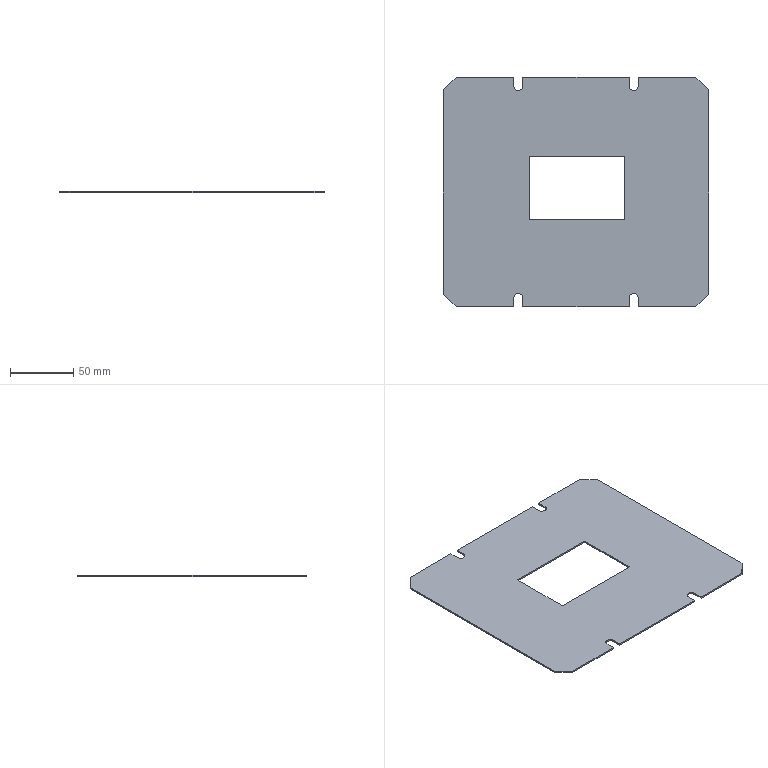Part | SolidWorks | features ICE 6, MoveFace 2, BaseBody 1, Chamfer 1 | 1 solid | 30 faces | box 209.129 x 181.357 x 1.2 mm | volume 40439 mm3 | plane 26 | cylinder 4 | commonest cylinder face diameters 7 x4
STEP:
#1=CARTESIAN_POINT('',(-1.05,15.678,0.));
#2=VERTEX_POINT('',#1);
#3=CARTESIAN_POINT('',(-1.05,15.678,-1.2));
#4=VERTEX_POINT('',#3);
#5=CARTESIAN_POINT('',(-1.05,15.678,188.123));
#6=DIRECTION('',(0.,0.,-1.));
#7=VECTOR('',#6,1000.);
#8=LINE('',#5,#7);
#9=EDGE_CURVE('',#2,#4,#8,.T.);
#10=ORIENTED_EDGE('',*,*,#9,.F.);
#11=CARTESIAN_POINT('',(44.565,15.678,0.));
#12=VERTEX_POINT('',#11);
#13=CARTESIAN_POINT('',(4.565,15.678,0.));
#14=DIRECTION('',(1.,0.,0.));
#15=VECTOR('',#14,1000.);
#16=LINE('',#13,#15);
#17=EDGE_CURVE('',#2,#12,#16,.T.);
#18=ORIENTED_EDGE('',*,*,#17,.T.);
#19=CARTESIAN_POINT('',(44.565,15.678,-1.2));
#20=VERTEX_POINT('',#19);
#21=CARTESIAN_POINT('',(44.565,15.678,188.123));
#22=DIRECTION('',(0.,0.,-1.));
#23=VECTOR('',#22,1000.);
#24=LINE('',#21,#23);
#25=EDGE_CURVE('',#12,#20,#24,.T.);
#26=ORIENTED_EDGE('',*,*,#25,.T.);
#27=CARTESIAN_POINT('',(122.729,15.678,-1.2));
#28=DIRECTION('',(1.,0.,0.));
#29=VECTOR('',#28,1000.);
#30=LINE('',#27,#29);
#31=EDGE_CURVE('',#4,#20,#30,.T.);
#32=ORIENTED_EDGE('',*,*,#31,.F.);
#33=EDGE_LOOP('',(#10,#18,#26,#32));
#34=FACE_OUTER_BOUND('',#33,.T.);
#35=CARTESIAN_POINT('',(4.565,15.678,188.123));
#36=DIRECTION('',(0.,1.,0.));
#37=DIRECTION('',(-1.,0.,0.));
#38=AXIS2_PLACEMENT_3D('',#35,#36,#37);
#39=PLANE('',#38);
#40=ADVANCED_FACE('',(#34),#39,.T.);
#41=CARTESIAN_POINT('',(-98.95,15.678,-1.2));
#42=VERTEX_POINT('',#41);
#43=CARTESIAN_POINT('',(-98.95,15.678,0.));
#44=VERTEX_POINT('',#43);
#45=CARTESIAN_POINT('',(-98.95,15.678,188.123));
#46=DIRECTION('',(0.,0.,1.));
#47=VECTOR('',#46,1000.);
#48=LINE('',#45,#47);
#49=EDGE_CURVE('',#42,#44,#48,.T.);
#50=ORIENTED_EDGE('',*,*,#49,.F.);
#51=CARTESIAN_POINT('',(-144.565,15.678,-1.2));
#52=VERTEX_POINT('',#51);
#53=CARTESIAN_POINT('',(122.729,15.678,-1.2));
#54=DIRECTION('',(1.,0.,0.));
#55=VECTOR('',#54,1000.);
#56=LINE('',#53,#55);
#57=EDGE_CURVE('',#52,#42,#56,.T.);
#58=ORIENTED_EDGE('',*,*,#57,.F.);
#59=CARTESIAN_POINT('',(-144.565,15.678,0.));
#60=VERTEX_POINT('',#59);
#61=CARTESIAN_POINT('',(-144.565,15.678,188.123));
#62=DIRECTION('',(0.,0.,1.));
#63=VECTOR('',#62,1000.);
#64=LINE('',#61,#63);
#65=EDGE_CURVE('',#52,#60,#64,.T.);
#66=ORIENTED_EDGE('',*,*,#65,.T.);
#67=CARTESIAN_POINT('',(4.565,15.678,0.));
#68=DIRECTION('',(1.,0.,0.));
#69=VECTOR('',#68,1000.);
#70=LINE('',#67,#69);
#71=EDGE_CURVE('',#60,#44,#70,.T.);
#72=ORIENTED_EDGE('',*,*,#71,.T.);
#73=EDGE_LOOP('',(#50,#58,#66,#72));
#74=FACE_OUTER_BOUND('',#73,.T.);
#75=CARTESIAN_POINT('',(4.565,15.678,188.123));
#76=DIRECTION('',(0.,1.,0.));
#77=DIRECTION('',(-1.,0.,0.));
#78=AXIS2_PLACEMENT_3D('',#75,#76,#77);
#79=PLANE('',#78);
#80=ADVANCED_FACE('',(#74),#79,.T.);
#81=CARTESIAN_POINT('',(-98.95,-165.678,0.));
#82=VERTEX_POINT('',#81);
#83=CARTESIAN_POINT('',(-98.95,-165.678,-1.2));
#84=VERTEX_POINT('',#83);
#85=CARTESIAN_POINT('',(-98.95,-165.678,188.123));
#86=DIRECTION('',(0.,0.,-1.));
#87=VECTOR('',#86,1000.);
#88=LINE('',#85,#87);
#89=EDGE_CURVE('',#82,#84,#88,.T.);
#90=ORIENTED_EDGE('',*,*,#89,.F.);
#91=CARTESIAN_POINT('',(-144.565,-165.678,0.));
#92=VERTEX_POINT('',#91);
#93=CARTESIAN_POINT('',(4.565,-165.678,0.));
#94=DIRECTION('',(-1.,0.,0.));
#95=VECTOR('',#94,1000.);
#96=LINE('',#93,#95);
#97=EDGE_CURVE('',#82,#92,#96,.T.);
#98=ORIENTED_EDGE('',*,*,#97,.T.);
#99=CARTESIAN_POINT('',(-144.565,-165.678,-1.2));
#100=VERTEX_POINT('',#99);
#101=CARTESIAN_POINT('',(-144.565,-165.678,188.123));
#102=DIRECTION('',(0.,0.,-1.));
#103=VECTOR('',#102,1000.);
#104=LINE('',#101,#103);
#105=EDGE_CURVE('',#92,#100,#104,.T.);
#106=ORIENTED_EDGE('',*,*,#105,.T.);
#107=CARTESIAN_POINT('',(-122.729,-165.678,-1.2));
#108=DIRECTION('',(-1.,0.,0.));
#109=VECTOR('',#108,1000.);
#110=LINE('',#107,#109);
#111=EDGE_CURVE('',#84,#100,#110,.T.);
#112=ORIENTED_EDGE('',*,*,#111,.F.);
#113=EDGE_LOOP('',(#90,#98,#106,#112));
#114=FACE_OUTER_BOUND('',#113,.T.);
#115=CARTESIAN_POINT('',(4.565,-165.678,188.123));
#116=DIRECTION('',(0.,-1.,0.));
#117=DIRECTION('',(1.,0.,0.));
#118=AXIS2_PLACEMENT_3D('',#115,#116,#117);
#119=PLANE('',#118);
#120=ADVANCED_FACE('',(#114),#119,.T.);
#121=CARTESIAN_POINT('',(-1.05,-165.678,-1.2));
#122=VERTEX_POINT('',#121);
#123=CARTESIAN_POINT('',(-1.05,-165.678,0.));
#124=VERTEX_POINT('',#123);
#125=CARTESIAN_POINT('',(-1.05,-165.678,188.123));
#126=DIRECTION('',(0.,0.,1.));
#127=VECTOR('',#126,1000.);
#128=LINE('',#125,#127);
#129=EDGE_CURVE('',#122,#124,#128,.T.);
#130=ORIENTED_EDGE('',*,*,#129,.F.);
#131=CARTESIAN_POINT('',(44.565,-165.678,-1.2));
#132=VERTEX_POINT('',#131);
#133=CARTESIAN_POINT('',(-122.729,-165.678,-1.2));
#134=DIRECTION('',(-1.,0.,0.));
#135=VECTOR('',#134,1000.);
#136=LINE('',#133,#135);
#137=EDGE_CURVE('',#132,#122,#136,.T.);
#138=ORIENTED_EDGE('',*,*,#137,.F.);
#139=CARTESIAN_POINT('',(44.565,-165.678,0.));
#140=VERTEX_POINT('',#139);
#141=CARTESIAN_POINT('',(44.565,-165.678,188.123));
#142=DIRECTION('',(0.,0.,1.));
#143=VECTOR('',#142,1000.);
#144=LINE('',#141,#143);
#145=EDGE_CURVE('',#132,#140,#144,.T.);
#146=ORIENTED_EDGE('',*,*,#145,.T.);
#147=CARTESIAN_POINT('',(4.565,-165.678,0.));
#148=DIRECTION('',(-1.,0.,0.));
#149=VECTOR('',#148,1000.);
#150=LINE('',#147,#149);
#151=EDGE_CURVE('',#140,#124,#150,.T.);
#152=ORIENTED_EDGE('',*,*,#151,.T.);
#153=EDGE_LOOP('',(#130,#138,#146,#152));
#154=FACE_OUTER_BOUND('',#153,.T.);
#155=CARTESIAN_POINT('',(4.565,-165.678,188.123));
#156=DIRECTION('',(0.,-1.,0.));
#157=DIRECTION('',(1.,0.,0.));
#158=AXIS2_PLACEMENT_3D('',#155,#156,#157);
#159=PLANE('',#158);
#160=ADVANCED_FACE('',(#154),#159,.T.);
#161=CARTESIAN_POINT('',(-87.,-46.7,0.));
#162=VERTEX_POINT('',#161);
#163=CARTESIAN_POINT('',(-87.,-96.7,0.));
#164=VERTEX_POINT('',#163);
#165=CARTESIAN_POINT('',(-87.,-46.7,0.));
#166=DIRECTION('',(0.,-1.,0.));
#167=VECTOR('',#166,1000.);
#168=LINE('',#165,#167);
#169=EDGE_CURVE('',#162,#164,#168,.T.);
#170=ORIENTED_EDGE('',*,*,#169,.F.);
#171=CARTESIAN_POINT('',(-12.,-46.7,0.));
#172=VERTEX_POINT('',#171);
#173=CARTESIAN_POINT('',(-87.,-46.7,0.));
#174=DIRECTION('',(-1.,0.,0.));
#175=VECTOR('',#174,1000.);
#176=LINE('',#173,#175);
#177=EDGE_CURVE('',#172,#162,#176,.T.);
#178=ORIENTED_EDGE('',*,*,#177,.F.);
#179=CARTESIAN_POINT('',(-12.,-96.7,0.));
#180=VERTEX_POINT('',#179);
#181=CARTESIAN_POINT('',(-12.,-46.7,0.));
#182=DIRECTION('',(0.,1.,0.));
#183=VECTOR('',#182,1000.);
#184=LINE('',#181,#183);
#185=EDGE_CURVE('',#180,#172,#184,.T.);
#186=ORIENTED_EDGE('',*,*,#185,.F.);
#187=CARTESIAN_POINT('',(-87.,-96.7,0.));
#188=DIRECTION('',(1.,0.,0.));
#189=VECTOR('',#188,1000.);
#190=LINE('',#187,#189);
#191=EDGE_CURVE('',#164,#180,#190,.T.);
#192=ORIENTED_EDGE('',*,*,#191,.F.);
#193=EDGE_LOOP('',(#170,#178,#186,#192));
#194=FACE_BOUND('',#193,.T.);
#195=ORIENTED_EDGE('',*,*,#17,.F.);
#196=CARTESIAN_POINT('',(-1.05,8.5,0.));
#197=VERTEX_POINT('',#196);
#198=CARTESIAN_POINT('',(-1.05,0.,0.));
#199=DIRECTION('',(0.,-1.,0.));
#200=VECTOR('',#199,1000.);
#201=LINE('',#198,#200);
#202=EDGE_CURVE('',#2,#197,#201,.T.);
#203=ORIENTED_EDGE('',*,*,#202,.T.);
#204=CARTESIAN_POINT('',(-8.05,8.5,0.));
#205=VERTEX_POINT('',#204);
#206=CARTESIAN_POINT('',(-4.55,8.5,0.));
#207=DIRECTION('',(0.,0.,-1.));
#208=DIRECTION('',(1.,0.,0.));
#209=AXIS2_PLACEMENT_3D('',#206,#207,#208);
#210=CIRCLE('',#209,3.5);
#211=EDGE_CURVE('',#197,#205,#210,.T.);
#212=ORIENTED_EDGE('',*,*,#211,.T.);
#213=CARTESIAN_POINT('',(-8.05,15.678,0.));
#214=VERTEX_POINT('',#213);
#215=CARTESIAN_POINT('',(-8.05,0.,0.));
#216=DIRECTION('',(0.,1.,0.));
#217=VECTOR('',#216,1000.);
#218=LINE('',#215,#217);
#219=EDGE_CURVE('',#205,#214,#218,.T.);
#220=ORIENTED_EDGE('',*,*,#219,.T.);
#221=CARTESIAN_POINT('',(-91.95,15.678,0.));
#222=VERTEX_POINT('',#221);
#223=CARTESIAN_POINT('',(4.565,15.678,0.));
#224=DIRECTION('',(1.,0.,0.));
#225=VECTOR('',#224,1000.);
#226=LINE('',#223,#225);
#227=EDGE_CURVE('',#222,#214,#226,.T.);
#228=ORIENTED_EDGE('',*,*,#227,.F.);
#229=CARTESIAN_POINT('',(-91.95,8.5,0.));
#230=VERTEX_POINT('',#229);
#231=CARTESIAN_POINT('',(-91.95,0.,0.));
#232=DIRECTION('',(0.,-1.,0.));
#233=VECTOR('',#232,1000.);
#234=LINE('',#231,#233);
#235=EDGE_CURVE('',#222,#230,#234,.T.);
#236=ORIENTED_EDGE('',*,*,#235,.T.);
#237=CARTESIAN_POINT('',(-98.95,8.5,0.));
#238=VERTEX_POINT('',#237);
#239=CARTESIAN_POINT('',(-95.45,8.5,0.));
#240=DIRECTION('',(0.,0.,-1.));
#241=DIRECTION('',(1.,0.,0.));
#242=AXIS2_PLACEMENT_3D('',#239,#240,#241);
#243=CIRCLE('',#242,3.5);
#244=EDGE_CURVE('',#230,#238,#243,.T.);
#245=ORIENTED_EDGE('',*,*,#244,.T.);
#246=CARTESIAN_POINT('',(-98.95,0.,0.));
#247=DIRECTION('',(0.,1.,0.));
#248=VECTOR('',#247,1000.);
#249=LINE('',#246,#248);
#250=EDGE_CURVE('',#238,#44,#249,.T.);
#251=ORIENTED_EDGE('',*,*,#250,.T.);
#252=ORIENTED_EDGE('',*,*,#71,.F.);
#253=CARTESIAN_POINT('',(-154.565,5.678,0.));
#254=VERTEX_POINT('',#253);
#255=CARTESIAN_POINT('',(-80.122,80.122,0.));
#256=DIRECTION('',(-0.7071,-0.7071,0.));
#257=VECTOR('',#256,1000.);
#258=LINE('',#255,#257);
#259=EDGE_CURVE('',#60,#254,#258,.T.);
#260=ORIENTED_EDGE('',*,*,#259,.T.);
#261=CARTESIAN_POINT('',(-154.565,-155.678,0.));
#262=VERTEX_POINT('',#261);
#263=CARTESIAN_POINT('',(-154.565,15.678,0.));
#264=DIRECTION('',(0.,1.,0.));
#265=VECTOR('',#264,1000.);
#266=LINE('',#263,#265);
#267=EDGE_CURVE('',#262,#254,#266,.T.);
#268=ORIENTED_EDGE('',*,*,#267,.F.);
#269=CARTESIAN_POINT('',(-155.122,-155.122,0.));
#270=DIRECTION('',(0.7071,-0.7071,0.));
#271=VECTOR('',#270,1000.);
#272=LINE('',#269,#271);
#273=EDGE_CURVE('',#262,#92,#272,.T.);
#274=ORIENTED_EDGE('',*,*,#273,.T.);
#275=ORIENTED_EDGE('',*,*,#97,.F.);
#276=CARTESIAN_POINT('',(-98.95,-158.5,0.));
#277=VERTEX_POINT('',#276);
#278=CARTESIAN_POINT('',(-98.95,0.,0.));
#279=DIRECTION('',(0.,1.,0.));
#280=VECTOR('',#279,1000.);
#281=LINE('',#278,#280);
#282=EDGE_CURVE('',#82,#277,#281,.T.);
#283=ORIENTED_EDGE('',*,*,#282,.T.);
#284=CARTESIAN_POINT('',(-91.95,-158.5,0.));
#285=VERTEX_POINT('',#284);
#286=CARTESIAN_POINT('',(-95.45,-158.5,0.));
#287=DIRECTION('',(0.,0.,-1.));
#288=DIRECTION('',(1.,0.,0.));
#289=AXIS2_PLACEMENT_3D('',#286,#287,#288);
#290=CIRCLE('',#289,3.5);
#291=EDGE_CURVE('',#277,#285,#290,.T.);
#292=ORIENTED_EDGE('',*,*,#291,.T.);
#293=CARTESIAN_POINT('',(-91.95,-165.678,0.));
#294=VERTEX_POINT('',#293);
#295=CARTESIAN_POINT('',(-91.95,0.,0.));
#296=DIRECTION('',(0.,-1.,0.));
#297=VECTOR('',#296,1000.);
#298=LINE('',#295,#297);
#299=EDGE_CURVE('',#285,#294,#298,.T.);
#300=ORIENTED_EDGE('',*,*,#299,.T.);
#301=CARTESIAN_POINT('',(-8.05,-165.678,0.));
#302=VERTEX_POINT('',#301);
#303=CARTESIAN_POINT('',(4.565,-165.678,0.));
#304=DIRECTION('',(-1.,0.,0.));
#305=VECTOR('',#304,1000.);
#306=LINE('',#303,#305);
#307=EDGE_CURVE('',#302,#294,#306,.T.);
#308=ORIENTED_EDGE('',*,*,#307,.F.);
#309=CARTESIAN_POINT('',(-8.05,-158.5,0.));
#310=VERTEX_POINT('',#309);
#311=CARTESIAN_POINT('',(-8.05,0.,0.));
#312=DIRECTION('',(0.,1.,0.));
#313=VECTOR('',#312,1000.);
#314=LINE('',#311,#313);
#315=EDGE_CURVE('',#302,#310,#314,.T.);
#316=ORIENTED_EDGE('',*,*,#315,.T.);
#317=CARTESIAN_POINT('',(-1.05,-158.5,0.));
#318=VERTEX_POINT('',#317);
#319=CARTESIAN_POINT('',(-4.55,-158.5,0.));
#320=DIRECTION('',(0.,0.,-1.));
#321=DIRECTION('',(1.,0.,0.));
#322=AXIS2_PLACEMENT_3D('',#319,#320,#321);
#323=CIRCLE('',#322,3.5);
#324=EDGE_CURVE('',#310,#318,#323,.T.);
#325=ORIENTED_EDGE('',*,*,#324,.T.);
#326=CARTESIAN_POINT('',(-1.05,0.,0.));
#327=DIRECTION('',(0.,-1.,0.));
#328=VECTOR('',#327,1000.);
#329=LINE('',#326,#328);
#330=EDGE_CURVE('',#318,#124,#329,.T.);
#331=ORIENTED_EDGE('',*,*,#330,.T.);
#332=ORIENTED_EDGE('',*,*,#151,.F.);
#333=CARTESIAN_POINT('',(54.565,-155.678,0.));
#334=VERTEX_POINT('',#333);
#335=CARTESIAN_POINT('',(105.122,-105.122,0.));
#336=DIRECTION('',(0.7071,0.7071,0.));
#337=VECTOR('',#336,1000.);
#338=LINE('',#335,#337);
#339=EDGE_CURVE('',#140,#334,#338,.T.);
#340=ORIENTED_EDGE('',*,*,#339,.T.);
#341=CARTESIAN_POINT('',(54.565,5.678,0.));
#342=VERTEX_POINT('',#341);
#343=CARTESIAN_POINT('',(54.565,15.678,0.));
#344=DIRECTION('',(0.,-1.,0.));
#345=VECTOR('',#344,1000.);
#346=LINE('',#343,#345);
#347=EDGE_CURVE('',#342,#334,#346,.T.);
#348=ORIENTED_EDGE('',*,*,#347,.F.);
#349=CARTESIAN_POINT('',(30.122,30.122,0.));
#350=DIRECTION('',(-0.7071,0.7071,0.));
#351=VECTOR('',#350,1000.);
#352=LINE('',#349,#351);
#353=EDGE_CURVE('',#342,#12,#352,.T.);
#354=ORIENTED_EDGE('',*,*,#353,.T.);
#355=EDGE_LOOP('',(#195,#203,#212,#220,#228,#236,#245,#251,#252,#260,#268,#274,#275,#283,#292,#300,#308,#316,#325,#331,#332,#340,#348,#354));
#356=FACE_OUTER_BOUND('',#355,.T.);
#357=CARTESIAN_POINT('',(0.,0.,0.));
#358=DIRECTION('',(0.,0.,1.));
#359=DIRECTION('',(1.,0.,0.));
#360=AXIS2_PLACEMENT_3D('',#357,#358,#359);
#361=PLANE('',#360);
#362=ADVANCED_FACE('',(#194,#356),#361,.T.);
#363=CARTESIAN_POINT('',(-1.05,-158.5,-1.2));
#364=VERTEX_POINT('',#363);
#365=CARTESIAN_POINT('',(-1.05,-158.5,-12.6));
#366=DIRECTION('',(0.,0.,1.));
#367=VECTOR('',#366,1000.);
#368=LINE('',#365,#367);
#369=EDGE_CURVE('',#364,#318,#368,.T.);
#370=ORIENTED_EDGE('',*,*,#369,.F.);
#371=CARTESIAN_POINT('',(-1.05,-173.5,-1.2));
#372=DIRECTION('',(0.,1.,0.));
#373=VECTOR('',#372,1000.);
#374=LINE('',#371,#373);
#375=EDGE_CURVE('',#122,#364,#374,.T.);
#376=ORIENTED_EDGE('',*,*,#375,.F.);
#377=ORIENTED_EDGE('',*,*,#129,.T.);
#378=ORIENTED_EDGE('',*,*,#330,.F.);
#379=EDGE_LOOP('',(#370,#376,#377,#378));
#380=FACE_OUTER_BOUND('',#379,.T.);
#381=CARTESIAN_POINT('',(-1.05,-173.5,-12.6));
#382=DIRECTION('',(1.,0.,0.));
#383=DIRECTION('',(0.,0.,-1.));
#384=AXIS2_PLACEMENT_3D('',#381,#382,#383);
#385=PLANE('',#384);
#386=ADVANCED_FACE('',(#380),#385,.F.);
#387=ORIENTED_EDGE('',*,*,#324,.F.);
#388=CARTESIAN_POINT('',(-8.05,-158.5,-1.2));
#389=VERTEX_POINT('',#388);
#390=CARTESIAN_POINT('',(-8.05,-158.5,-12.6));
#391=DIRECTION('',(0.,0.,1.));
#392=VECTOR('',#391,1000.);
#393=LINE('',#390,#392);
#394=EDGE_CURVE('',#389,#310,#393,.T.);
#395=ORIENTED_EDGE('',*,*,#394,.F.);
#396=CARTESIAN_POINT('',(-4.55,-158.5,-1.2));
#397=DIRECTION('',(0.,0.,1.));
#398=DIRECTION('',(1.,0.,0.));
#399=AXIS2_PLACEMENT_3D('',#396,#397,#398);
#400=CIRCLE('',#399,3.5);
#401=EDGE_CURVE('',#364,#389,#400,.T.);
#402=ORIENTED_EDGE('',*,*,#401,.F.);
#403=ORIENTED_EDGE('',*,*,#369,.T.);
#404=EDGE_LOOP('',(#387,#395,#402,#403));
#405=FACE_OUTER_BOUND('',#404,.T.);
#406=CARTESIAN_POINT('',(-4.55,-158.5,-12.6));
#407=DIRECTION('',(0.,0.,1.));
#408=DIRECTION('',(1.,0.,0.));
#409=AXIS2_PLACEMENT_3D('',#406,#407,#408);
#410=CYLINDRICAL_SURFACE('',#409,3.5);
#411=ADVANCED_FACE('',(#405),#410,.F.);
#412=ORIENTED_EDGE('',*,*,#315,.F.);
#413=CARTESIAN_POINT('',(-8.05,-165.678,-1.2));
#414=VERTEX_POINT('',#413);
#415=CARTESIAN_POINT('',(-8.05,-165.678,188.123));
#416=DIRECTION('',(0.,0.,-1.));
#417=VECTOR('',#416,1000.);
#418=LINE('',#415,#417);
#419=EDGE_CURVE('',#302,#414,#418,.T.);
#420=ORIENTED_EDGE('',*,*,#419,.T.);
#421=CARTESIAN_POINT('',(-8.05,-173.5,-1.2));
#422=DIRECTION('',(0.,-1.,0.));
#423=VECTOR('',#422,1000.);
#424=LINE('',#421,#423);
#425=EDGE_CURVE('',#389,#414,#424,.T.);
#426=ORIENTED_EDGE('',*,*,#425,.F.);
#427=ORIENTED_EDGE('',*,*,#394,.T.);
#428=EDGE_LOOP('',(#412,#420,#426,#427));
#429=FACE_OUTER_BOUND('',#428,.T.);
#430=CARTESIAN_POINT('',(-8.05,-173.5,-12.6));
#431=DIRECTION('',(-1.,0.,0.));
#432=DIRECTION('',(0.,0.,1.));
#433=AXIS2_PLACEMENT_3D('',#430,#431,#432);
#434=PLANE('',#433);
#435=ADVANCED_FACE('',(#429),#434,.F.);
#436=CARTESIAN_POINT('',(-91.95,-158.5,-1.2));
#437=VERTEX_POINT('',#436);
#438=CARTESIAN_POINT('',(-91.95,-158.5,-12.6));
#439=DIRECTION('',(0.,0.,1.));
#440=VECTOR('',#439,1000.);
#441=LINE('',#438,#440);
#442=EDGE_CURVE('',#437,#285,#441,.T.);
#443=ORIENTED_EDGE('',*,*,#442,.F.);
#444=CARTESIAN_POINT('',(-91.95,-165.678,-1.2));
#445=VERTEX_POINT('',#444);
#446=CARTESIAN_POINT('',(-91.95,-173.5,-1.2));
#447=DIRECTION('',(0.,1.,0.));
#448=VECTOR('',#447,1000.);
#449=LINE('',#446,#448);
#450=EDGE_CURVE('',#445,#437,#449,.T.);
#451=ORIENTED_EDGE('',*,*,#450,.F.);
#452=CARTESIAN_POINT('',(-91.95,-165.678,188.123));
#453=DIRECTION('',(0.,0.,1.));
#454=VECTOR('',#453,1000.);
#455=LINE('',#452,#454);
#456=EDGE_CURVE('',#445,#294,#455,.T.);
#457=ORIENTED_EDGE('',*,*,#456,.T.);
#458=ORIENTED_EDGE('',*,*,#299,.F.);
#459=EDGE_LOOP('',(#443,#451,#457,#458));
#460=FACE_OUTER_BOUND('',#459,.T.);
#461=CARTESIAN_POINT('',(-91.95,-173.5,-12.6));
#462=DIRECTION('',(1.,0.,0.));
#463=DIRECTION('',(0.,0.,-1.));
#464=AXIS2_PLACEMENT_3D('',#461,#462,#463);
#465=PLANE('',#464);
#466=ADVANCED_FACE('',(#460),#465,.F.);
#467=ORIENTED_EDGE('',*,*,#291,.F.);
#468=CARTESIAN_POINT('',(-98.95,-158.5,-1.2));
#469=VERTEX_POINT('',#468);
#470=CARTESIAN_POINT('',(-98.95,-158.5,-12.6));
#471=DIRECTION('',(0.,0.,1.));
#472=VECTOR('',#471,1000.);
#473=LINE('',#470,#472);
#474=EDGE_CURVE('',#469,#277,#473,.T.);
#475=ORIENTED_EDGE('',*,*,#474,.F.);
#476=CARTESIAN_POINT('',(-95.45,-158.5,-1.2));
#477=DIRECTION('',(0.,0.,1.));
#478=DIRECTION('',(1.,0.,0.));
#479=AXIS2_PLACEMENT_3D('',#476,#477,#478);
#480=CIRCLE('',#479,3.5);
#481=EDGE_CURVE('',#437,#469,#480,.T.);
#482=ORIENTED_EDGE('',*,*,#481,.F.);
#483=ORIENTED_EDGE('',*,*,#442,.T.);
#484=EDGE_LOOP('',(#467,#475,#482,#483));
#485=FACE_OUTER_BOUND('',#484,.T.);
#486=CARTESIAN_POINT('',(-95.45,-158.5,-12.6));
#487=DIRECTION('',(0.,0.,1.));
#488=DIRECTION('',(1.,0.,0.));
#489=AXIS2_PLACEMENT_3D('',#486,#487,#488);
#490=CYLINDRICAL_SURFACE('',#489,3.5);
#491=ADVANCED_FACE('',(#485),#490,.F.);
#492=ORIENTED_EDGE('',*,*,#282,.F.);
#493=ORIENTED_EDGE('',*,*,#89,.T.);
#494=CARTESIAN_POINT('',(-98.95,-173.5,-1.2));
#495=DIRECTION('',(0.,-1.,0.));
#496=VECTOR('',#495,1000.);
#497=LINE('',#494,#496);
#498=EDGE_CURVE('',#469,#84,#497,.T.);
#499=ORIENTED_EDGE('',*,*,#498,.F.);
#500=ORIENTED_EDGE('',*,*,#474,.T.);
#501=EDGE_LOOP('',(#492,#493,#499,#500));
#502=FACE_OUTER_BOUND('',#501,.T.);
#503=CARTESIAN_POINT('',(-98.95,-173.5,-12.6));
#504=DIRECTION('',(-1.,0.,0.));
#505=DIRECTION('',(0.,0.,1.));
#506=AXIS2_PLACEMENT_3D('',#503,#504,#505);
#507=PLANE('',#506);
#508=ADVANCED_FACE('',(#502),#507,.F.);
#509=CARTESIAN_POINT('',(-98.95,8.5,-1.2));
#510=VERTEX_POINT('',#509);
#511=CARTESIAN_POINT('',(-98.95,8.5,-12.6));
#512=DIRECTION('',(0.,0.,1.));
#513=VECTOR('',#512,1000.);
#514=LINE('',#511,#513);
#515=EDGE_CURVE('',#510,#238,#514,.T.);
#516=ORIENTED_EDGE('',*,*,#515,.F.);
#517=CARTESIAN_POINT('',(-98.95,173.5,-1.2));
#518=DIRECTION('',(0.,-1.,0.));
#519=VECTOR('',#518,1000.);
#520=LINE('',#517,#519);
#521=EDGE_CURVE('',#42,#510,#520,.T.);
#522=ORIENTED_EDGE('',*,*,#521,.F.);
#523=ORIENTED_EDGE('',*,*,#49,.T.);
#524=ORIENTED_EDGE('',*,*,#250,.F.);
#525=EDGE_LOOP('',(#516,#522,#523,#524));
#526=FACE_OUTER_BOUND('',#525,.T.);
#527=CARTESIAN_POINT('',(-98.95,173.5,-12.6));
#528=DIRECTION('',(-1.,0.,0.));
#529=DIRECTION('',(0.,0.,1.));
#530=AXIS2_PLACEMENT_3D('',#527,#528,#529);
#531=PLANE('',#530);
#532=ADVANCED_FACE('',(#526),#531,.F.);
#533=ORIENTED_EDGE('',*,*,#244,.F.);
#534=CARTESIAN_POINT('',(-91.95,8.5,-1.2));
#535=VERTEX_POINT('',#534);
#536=CARTESIAN_POINT('',(-91.95,8.5,-12.6));
#537=DIRECTION('',(0.,0.,1.));
#538=VECTOR('',#537,1000.);
#539=LINE('',#536,#538);
#540=EDGE_CURVE('',#535,#230,#539,.T.);
#541=ORIENTED_EDGE('',*,*,#540,.F.);
#542=CARTESIAN_POINT('',(-95.45,8.5,-1.2));
#543=DIRECTION('',(0.,0.,1.));
#544=DIRECTION('',(1.,0.,0.));
#545=AXIS2_PLACEMENT_3D('',#542,#543,#544);
#546=CIRCLE('',#545,3.5);
#547=EDGE_CURVE('',#510,#535,#546,.T.);
#548=ORIENTED_EDGE('',*,*,#547,.F.);
#549=ORIENTED_EDGE('',*,*,#515,.T.);
#550=EDGE_LOOP('',(#533,#541,#548,#549));
#551=FACE_OUTER_BOUND('',#550,.T.);
#552=CARTESIAN_POINT('',(-95.45,8.5,-12.6));
#553=DIRECTION('',(0.,0.,1.));
#554=DIRECTION('',(1.,0.,0.));
#555=AXIS2_PLACEMENT_3D('',#552,#553,#554);
#556=CYLINDRICAL_SURFACE('',#555,3.5);
#557=ADVANCED_FACE('',(#551),#556,.F.);
#558=ORIENTED_EDGE('',*,*,#235,.F.);
#559=CARTESIAN_POINT('',(-91.95,15.678,-1.2));
#560=VERTEX_POINT('',#559);
#561=CARTESIAN_POINT('',(-91.95,15.678,188.123));
#562=DIRECTION('',(0.,0.,-1.));
#563=VECTOR('',#562,1000.);
#564=LINE('',#561,#563);
#565=EDGE_CURVE('',#222,#560,#564,.T.);
#566=ORIENTED_EDGE('',*,*,#565,.T.);
#567=CARTESIAN_POINT('',(-91.95,173.5,-1.2));
#568=DIRECTION('',(0.,1.,0.));
#569=VECTOR('',#568,1000.);
#570=LINE('',#567,#569);
#571=EDGE_CURVE('',#535,#560,#570,.T.);
#572=ORIENTED_EDGE('',*,*,#571,.F.);
#573=ORIENTED_EDGE('',*,*,#540,.T.);
#574=EDGE_LOOP('',(#558,#566,#572,#573));
#575=FACE_OUTER_BOUND('',#574,.T.);
#576=CARTESIAN_POINT('',(-91.95,173.5,-12.6));
#577=DIRECTION('',(1.,0.,0.));
#578=DIRECTION('',(0.,0.,-1.));
#579=AXIS2_PLACEMENT_3D('',#576,#577,#578);
#580=PLANE('',#579);
#581=ADVANCED_FACE('',(#575),#580,.F.);
#582=CARTESIAN_POINT('',(-8.05,8.5,-1.2));
#583=VERTEX_POINT('',#582);
#584=CARTESIAN_POINT('',(-8.05,8.5,-12.6));
#585=DIRECTION('',(0.,0.,1.));
#586=VECTOR('',#585,1000.);
#587=LINE('',#584,#586);
#588=EDGE_CURVE('',#583,#205,#587,.T.);
#589=ORIENTED_EDGE('',*,*,#588,.F.);
#590=CARTESIAN_POINT('',(-8.05,15.678,-1.2));
#591=VERTEX_POINT('',#590);
#592=CARTESIAN_POINT('',(-8.05,173.5,-1.2));
#593=DIRECTION('',(0.,-1.,0.));
#594=VECTOR('',#593,1000.);
#595=LINE('',#592,#594);
#596=EDGE_CURVE('',#591,#583,#595,.T.);
#597=ORIENTED_EDGE('',*,*,#596,.F.);
#598=CARTESIAN_POINT('',(-8.05,15.678,188.123));
#599=DIRECTION('',(0.,0.,1.));
#600=VECTOR('',#599,1000.);
#601=LINE('',#598,#600);
#602=EDGE_CURVE('',#591,#214,#601,.T.);
#603=ORIENTED_EDGE('',*,*,#602,.T.);
#604=ORIENTED_EDGE('',*,*,#219,.F.);
#605=EDGE_LOOP('',(#589,#597,#603,#604));
#606=FACE_OUTER_BOUND('',#605,.T.);
#607=CARTESIAN_POINT('',(-8.05,173.5,-12.6));
#608=DIRECTION('',(-1.,0.,0.));
#609=DIRECTION('',(0.,0.,1.));
#610=AXIS2_PLACEMENT_3D('',#607,#608,#609);
#611=PLANE('',#610);
#612=ADVANCED_FACE('',(#606),#611,.F.);
#613=ORIENTED_EDGE('',*,*,#211,.F.);
#614=CARTESIAN_POINT('',(-1.05,8.5,-1.2));
#615=VERTEX_POINT('',#614);
#616=CARTESIAN_POINT('',(-1.05,8.5,-12.6));
#617=DIRECTION('',(0.,0.,1.));
#618=VECTOR('',#617,1000.);
#619=LINE('',#616,#618);
#620=EDGE_CURVE('',#615,#197,#619,.T.);
#621=ORIENTED_EDGE('',*,*,#620,.F.);
#622=CARTESIAN_POINT('',(-4.55,8.5,-1.2));
#623=DIRECTION('',(0.,0.,1.));
#624=DIRECTION('',(1.,0.,0.));
#625=AXIS2_PLACEMENT_3D('',#622,#623,#624);
#626=CIRCLE('',#625,3.5);
#627=EDGE_CURVE('',#583,#615,#626,.T.);
#628=ORIENTED_EDGE('',*,*,#627,.F.);
#629=ORIENTED_EDGE('',*,*,#588,.T.);
#630=EDGE_LOOP('',(#613,#621,#628,#629));
#631=FACE_OUTER_BOUND('',#630,.T.);
#632=CARTESIAN_POINT('',(-4.55,8.5,-12.6));
#633=DIRECTION('',(0.,0.,1.));
#634=DIRECTION('',(1.,0.,0.));
#635=AXIS2_PLACEMENT_3D('',#632,#633,#634);
#636=CYLINDRICAL_SURFACE('',#635,3.5);
#637=ADVANCED_FACE('',(#631),#636,.F.);
#638=ORIENTED_EDGE('',*,*,#202,.F.);
#639=ORIENTED_EDGE('',*,*,#9,.T.);
#640=CARTESIAN_POINT('',(-1.05,173.5,-1.2));
#641=DIRECTION('',(0.,1.,0.));
#642=VECTOR('',#641,1000.);
#643=LINE('',#640,#642);
#644=EDGE_CURVE('',#615,#4,#643,.T.);
#645=ORIENTED_EDGE('',*,*,#644,.F.);
#646=ORIENTED_EDGE('',*,*,#620,.T.);
#647=EDGE_LOOP('',(#638,#639,#645,#646));
#648=FACE_OUTER_BOUND('',#647,.T.);
#649=CARTESIAN_POINT('',(-1.05,173.5,-12.6));
#650=DIRECTION('',(1.,0.,0.));
#651=DIRECTION('',(0.,0.,-1.));
#652=AXIS2_PLACEMENT_3D('',#649,#650,#651);
#653=PLANE('',#652);
#654=ADVANCED_FACE('',(#648),#653,.F.);
#655=CARTESIAN_POINT('',(-12.,-46.7,-1.2));
#656=VERTEX_POINT('',#655);
#657=CARTESIAN_POINT('',(-87.,-46.7,-1.2));
#658=VERTEX_POINT('',#657);
#659=CARTESIAN_POINT('',(-87.,-46.7,-1.2));
#660=DIRECTION('',(-1.,0.,0.));
#661=VECTOR('',#660,1000.);
#662=LINE('',#659,#661);
#663=EDGE_CURVE('',#656,#658,#662,.T.);
#664=ORIENTED_EDGE('',*,*,#663,.T.);
#665=CARTESIAN_POINT('',(-87.,-96.7,-1.2));
#666=VERTEX_POINT('',#665);
#667=CARTESIAN_POINT('',(-87.,-46.7,-1.2));
#668=DIRECTION('',(0.,-1.,0.));
#669=VECTOR('',#668,1000.);
#670=LINE('',#667,#669);
#671=EDGE_CURVE('',#658,#666,#670,.T.);
#672=ORIENTED_EDGE('',*,*,#671,.T.);
#673=CARTESIAN_POINT('',(-12.,-96.7,-1.2));
#674=VERTEX_POINT('',#673);
#675=CARTESIAN_POINT('',(-87.,-96.7,-1.2));
#676=DIRECTION('',(1.,0.,0.));
#677=VECTOR('',#676,1000.);
#678=LINE('',#675,#677);
#679=EDGE_CURVE('',#666,#674,#678,.T.);
#680=ORIENTED_EDGE('',*,*,#679,.T.);
#681=CARTESIAN_POINT('',(-12.,-46.7,-1.2));
#682=DIRECTION('',(0.,1.,0.));
#683=VECTOR('',#682,1000.);
#684=LINE('',#681,#683);
#685=EDGE_CURVE('',#674,#656,#684,.T.);
#686=ORIENTED_EDGE('',*,*,#685,.T.);
#687=EDGE_LOOP('',(#664,#672,#680,#686));
#688=FACE_BOUND('',#687,.T.);
#689=ORIENTED_EDGE('',*,*,#111,.T.);
#690=CARTESIAN_POINT('',(-154.565,-155.678,-1.2));
#691=VERTEX_POINT('',#690);
#692=CARTESIAN_POINT('',(-144.565,-165.678,-1.2));
#693=DIRECTION('',(-0.7071,0.7071,0.));
#694=VECTOR('',#693,1000.);
#695=LINE('',#692,#694);
#696=EDGE_CURVE('',#100,#691,#695,.T.);
#697=ORIENTED_EDGE('',*,*,#696,.T.);
#698=CARTESIAN_POINT('',(-154.565,5.678,-1.2));
#699=VERTEX_POINT('',#698);
#700=CARTESIAN_POINT('',(-154.565,15.678,-1.2));
#701=DIRECTION('',(0.,1.,0.));
#702=VECTOR('',#701,1000.);
#703=LINE('',#700,#702);
#704=EDGE_CURVE('',#691,#699,#703,.T.);
#705=ORIENTED_EDGE('',*,*,#704,.T.);
#706=CARTESIAN_POINT('',(-154.565,5.678,-1.2));
#707=DIRECTION('',(0.7071,0.7071,0.));
#708=VECTOR('',#707,1000.);
#709=LINE('',#706,#708);
#710=EDGE_CURVE('',#699,#52,#709,.T.);
#711=ORIENTED_EDGE('',*,*,#710,.T.);
#712=ORIENTED_EDGE('',*,*,#57,.T.);
#713=ORIENTED_EDGE('',*,*,#521,.T.);
#714=ORIENTED_EDGE('',*,*,#547,.T.);
#715=ORIENTED_EDGE('',*,*,#571,.T.);
#716=CARTESIAN_POINT('',(122.729,15.678,-1.2));
#717=DIRECTION('',(1.,0.,0.));
#718=VECTOR('',#717,1000.);
#719=LINE('',#716,#718);
#720=EDGE_CURVE('',#560,#591,#719,.T.);
#721=ORIENTED_EDGE('',*,*,#720,.T.);
#722=ORIENTED_EDGE('',*,*,#596,.T.);
#723=ORIENTED_EDGE('',*,*,#627,.T.);
#724=ORIENTED_EDGE('',*,*,#644,.T.);
#725=ORIENTED_EDGE('',*,*,#31,.T.);
#726=CARTESIAN_POINT('',(54.565,5.678,-1.2));
#727=VERTEX_POINT('',#726);
#728=CARTESIAN_POINT('',(44.565,15.678,-1.2));
#729=DIRECTION('',(0.7071,-0.7071,0.));
#730=VECTOR('',#729,1000.);
#731=LINE('',#728,#730);
#732=EDGE_CURVE('',#20,#727,#731,.T.);
#733=ORIENTED_EDGE('',*,*,#732,.T.);
#734=CARTESIAN_POINT('',(54.565,-155.678,-1.2));
#735=VERTEX_POINT('',#734);
#736=CARTESIAN_POINT('',(54.565,15.678,-1.2));
#737=DIRECTION('',(0.,-1.,0.));
#738=VECTOR('',#737,1000.);
#739=LINE('',#736,#738);
#740=EDGE_CURVE('',#727,#735,#739,.T.);
#741=ORIENTED_EDGE('',*,*,#740,.T.);
#742=CARTESIAN_POINT('',(54.565,-155.678,-1.2));
#743=DIRECTION('',(-0.7071,-0.7071,0.));
#744=VECTOR('',#743,1000.);
#745=LINE('',#742,#744);
#746=EDGE_CURVE('',#735,#132,#745,.T.);
#747=ORIENTED_EDGE('',*,*,#746,.T.);
#748=ORIENTED_EDGE('',*,*,#137,.T.);
#749=ORIENTED_EDGE('',*,*,#375,.T.);
#750=ORIENTED_EDGE('',*,*,#401,.T.);
#751=ORIENTED_EDGE('',*,*,#425,.T.);
#752=CARTESIAN_POINT('',(-122.729,-165.678,-1.2));
#753=DIRECTION('',(-1.,0.,0.));
#754=VECTOR('',#753,1000.);
#755=LINE('',#752,#754);
#756=EDGE_CURVE('',#414,#445,#755,.T.);
#757=ORIENTED_EDGE('',*,*,#756,.T.);
#758=ORIENTED_EDGE('',*,*,#450,.T.);
#759=ORIENTED_EDGE('',*,*,#481,.T.);
#760=ORIENTED_EDGE('',*,*,#498,.T.);
#761=EDGE_LOOP('',(#689,#697,#705,#711,#712,#713,#714,#715,#721,#722,#723,#724,#725,#733,#741,#747,#748,#749,#750,#751,#757,#758,#759,#760));
#762=FACE_OUTER_BOUND('',#761,.T.);
#763=CARTESIAN_POINT('',(0.,0.,-1.2));
#764=DIRECTION('',(0.,0.,1.));
#765=DIRECTION('',(1.,0.,0.));
#766=AXIS2_PLACEMENT_3D('',#763,#764,#765);
#767=PLANE('',#766);
#768=ADVANCED_FACE('',(#688,#762),#767,.F.);
#769=ORIENTED_EDGE('',*,*,#602,.F.);
#770=ORIENTED_EDGE('',*,*,#720,.F.);
#771=ORIENTED_EDGE('',*,*,#565,.F.);
#772=ORIENTED_EDGE('',*,*,#227,.T.);
#773=EDGE_LOOP('',(#769,#770,#771,#772));
#774=FACE_OUTER_BOUND('',#773,.T.);
#775=CARTESIAN_POINT('',(4.565,15.678,188.123));
#776=DIRECTION('',(0.,1.,0.));
#777=DIRECTION('',(-1.,0.,0.));
#778=AXIS2_PLACEMENT_3D('',#775,#776,#777);
#779=PLANE('',#778);
#780=ADVANCED_FACE('',(#774),#779,.T.);
#781=ORIENTED_EDGE('',*,*,#347,.T.);
#782=CARTESIAN_POINT('',(54.565,-155.678,188.123));
#783=DIRECTION('',(0.,0.,-1.));
#784=VECTOR('',#783,1000.);
#785=LINE('',#782,#784);
#786=EDGE_CURVE('',#334,#735,#785,.T.);
#787=ORIENTED_EDGE('',*,*,#786,.T.);
#788=ORIENTED_EDGE('',*,*,#740,.F.);
#789=CARTESIAN_POINT('',(54.565,5.678,188.123));
#790=DIRECTION('',(0.,0.,1.));
#791=VECTOR('',#790,1000.);
#792=LINE('',#789,#791);
#793=EDGE_CURVE('',#727,#342,#792,.T.);
#794=ORIENTED_EDGE('',*,*,#793,.T.);
#795=EDGE_LOOP('',(#781,#787,#788,#794));
#796=FACE_OUTER_BOUND('',#795,.T.);
#797=CARTESIAN_POINT('',(54.565,15.678,188.123));
#798=DIRECTION('',(1.,0.,0.));
#799=DIRECTION('',(0.,1.,0.));
#800=AXIS2_PLACEMENT_3D('',#797,#798,#799);
#801=PLANE('',#800);
#802=ADVANCED_FACE('',(#796),#801,.T.);
#803=ORIENTED_EDGE('',*,*,#456,.F.);
#804=ORIENTED_EDGE('',*,*,#756,.F.);
#805=ORIENTED_EDGE('',*,*,#419,.F.);
#806=ORIENTED_EDGE('',*,*,#307,.T.);
#807=EDGE_LOOP('',(#803,#804,#805,#806));
#808=FACE_OUTER_BOUND('',#807,.T.);
#809=CARTESIAN_POINT('',(4.565,-165.678,188.123));
#810=DIRECTION('',(0.,-1.,0.));
#811=DIRECTION('',(1.,0.,0.));
#812=AXIS2_PLACEMENT_3D('',#809,#810,#811);
#813=PLANE('',#812);
#814=ADVANCED_FACE('',(#808),#813,.T.);
#815=ORIENTED_EDGE('',*,*,#704,.F.);
#816=CARTESIAN_POINT('',(-154.565,-155.678,188.123));
#817=DIRECTION('',(0.,0.,1.));
#818=VECTOR('',#817,1000.);
#819=LINE('',#816,#818);
#820=EDGE_CURVE('',#691,#262,#819,.T.);
#821=ORIENTED_EDGE('',*,*,#820,.T.);
#822=ORIENTED_EDGE('',*,*,#267,.T.);
#823=CARTESIAN_POINT('',(-154.565,5.678,188.123));
#824=DIRECTION('',(0.,0.,-1.));
#825=VECTOR('',#824,1000.);
#826=LINE('',#823,#825);
#827=EDGE_CURVE('',#254,#699,#826,.T.);
#828=ORIENTED_EDGE('',*,*,#827,.T.);
#829=EDGE_LOOP('',(#815,#821,#822,#828));
#830=FACE_OUTER_BOUND('',#829,.T.);
#831=CARTESIAN_POINT('',(-154.565,15.678,188.123));
#832=DIRECTION('',(-1.,0.,0.));
#833=DIRECTION('',(0.,-1.,0.));
#834=AXIS2_PLACEMENT_3D('',#831,#832,#833);
#835=PLANE('',#834);
#836=ADVANCED_FACE('',(#830),#835,.T.);
#837=ORIENTED_EDGE('',*,*,#273,.F.);
#838=ORIENTED_EDGE('',*,*,#820,.F.);
#839=ORIENTED_EDGE('',*,*,#696,.F.);
#840=ORIENTED_EDGE('',*,*,#105,.F.);
#841=EDGE_LOOP('',(#837,#838,#839,#840));
#842=FACE_OUTER_BOUND('',#841,.T.);
#843=CARTESIAN_POINT('',(-144.565,-165.678,188.123));
#844=DIRECTION('',(0.7071,0.7071,0.));
#845=DIRECTION('',(0.,0.,-1.));
#846=AXIS2_PLACEMENT_3D('',#843,#844,#845);
#847=PLANE('',#846);
#848=ADVANCED_FACE('',(#842),#847,.F.);
#849=ORIENTED_EDGE('',*,*,#339,.F.);
#850=ORIENTED_EDGE('',*,*,#145,.F.);
#851=ORIENTED_EDGE('',*,*,#746,.F.);
#852=ORIENTED_EDGE('',*,*,#786,.F.);
#853=EDGE_LOOP('',(#849,#850,#851,#852));
#854=FACE_OUTER_BOUND('',#853,.T.);
#855=CARTESIAN_POINT('',(54.565,-155.678,188.123));
#856=DIRECTION('',(-0.7071,0.7071,0.));
#857=DIRECTION('',(0.,0.,-1.));
#858=AXIS2_PLACEMENT_3D('',#855,#856,#857);
#859=PLANE('',#858);
#860=ADVANCED_FACE('',(#854),#859,.F.);
#861=ORIENTED_EDGE('',*,*,#353,.F.);
#862=ORIENTED_EDGE('',*,*,#793,.F.);
#863=ORIENTED_EDGE('',*,*,#732,.F.);
#864=ORIENTED_EDGE('',*,*,#25,.F.);
#865=EDGE_LOOP('',(#861,#862,#863,#864));
#866=FACE_OUTER_BOUND('',#865,.T.);
#867=CARTESIAN_POINT('',(44.565,15.678,188.123));
#868=DIRECTION('',(-0.7071,-0.7071,0.));
#869=DIRECTION('',(0.,0.,-1.));
#870=AXIS2_PLACEMENT_3D('',#867,#868,#869);
#871=PLANE('',#870);
#872=ADVANCED_FACE('',(#866),#871,.F.);
#873=ORIENTED_EDGE('',*,*,#259,.F.);
#874=ORIENTED_EDGE('',*,*,#65,.F.);
#875=ORIENTED_EDGE('',*,*,#710,.F.);
#876=ORIENTED_EDGE('',*,*,#827,.F.);
#877=EDGE_LOOP('',(#873,#874,#875,#876));
#878=FACE_OUTER_BOUND('',#877,.T.);
#879=CARTESIAN_POINT('',(-154.565,5.678,188.123));
#880=DIRECTION('',(0.7071,-0.7071,0.));
#881=DIRECTION('',(0.,0.,-1.));
#882=AXIS2_PLACEMENT_3D('',#879,#880,#881);
#883=PLANE('',#882);
#884=ADVANCED_FACE('',(#878),#883,.F.);
#885=ORIENTED_EDGE('',*,*,#169,.T.);
#886=CARTESIAN_POINT('',(-87.,-96.7,-1.2));
#887=DIRECTION('',(0.,0.,1.));
#888=VECTOR('',#887,1000.);
#889=LINE('',#886,#888);
#890=EDGE_CURVE('',#666,#164,#889,.T.);
#891=ORIENTED_EDGE('',*,*,#890,.F.);
#892=ORIENTED_EDGE('',*,*,#671,.F.);
#893=CARTESIAN_POINT('',(-87.,-46.7,-1.2));
#894=DIRECTION('',(0.,0.,1.));
#895=VECTOR('',#894,1000.);
#896=LINE('',#893,#895);
#897=EDGE_CURVE('',#658,#162,#896,.T.);
#898=ORIENTED_EDGE('',*,*,#897,.T.);
#899=EDGE_LOOP('',(#885,#891,#892,#898));
#900=FACE_OUTER_BOUND('',#899,.T.);
#901=CARTESIAN_POINT('',(-87.,-46.7,-1.2));
#902=DIRECTION('',(-1.,0.,0.));
#903=DIRECTION('',(0.,0.,1.));
#904=AXIS2_PLACEMENT_3D('',#901,#902,#903);
#905=PLANE('',#904);
#906=ADVANCED_FACE('',(#900),#905,.F.);
#907=ORIENTED_EDGE('',*,*,#177,.T.);
#908=ORIENTED_EDGE('',*,*,#897,.F.);
#909=ORIENTED_EDGE('',*,*,#663,.F.);
#910=CARTESIAN_POINT('',(-12.,-46.7,-1.2));
#911=DIRECTION('',(0.,0.,1.));
#912=VECTOR('',#911,1000.);
#913=LINE('',#910,#912);
#914=EDGE_CURVE('',#656,#172,#913,.T.);
#915=ORIENTED_EDGE('',*,*,#914,.T.);
#916=EDGE_LOOP('',(#907,#908,#909,#915));
#917=FACE_OUTER_BOUND('',#916,.T.);
#918=CARTESIAN_POINT('',(-87.,-46.7,-1.2));
#919=DIRECTION('',(0.,1.,0.));
#920=DIRECTION('',(0.,0.,1.));
#921=AXIS2_PLACEMENT_3D('',#918,#919,#920);
#922=PLANE('',#921);
#923=ADVANCED_FACE('',(#917),#922,.F.);
#924=ORIENTED_EDGE('',*,*,#185,.T.);
#925=ORIENTED_EDGE('',*,*,#914,.F.);
#926=ORIENTED_EDGE('',*,*,#685,.F.);
#927=CARTESIAN_POINT('',(-12.,-96.7,-1.2));
#928=DIRECTION('',(0.,0.,1.));
#929=VECTOR('',#928,1000.);
#930=LINE('',#927,#929);
#931=EDGE_CURVE('',#674,#180,#930,.T.);
#932=ORIENTED_EDGE('',*,*,#931,.T.);
#933=EDGE_LOOP('',(#924,#925,#926,#932));
#934=FACE_OUTER_BOUND('',#933,.T.);
#935=CARTESIAN_POINT('',(-12.,-46.7,-1.2));
#936=DIRECTION('',(1.,0.,0.));
#937=DIRECTION('',(0.,1.,0.));
#938=AXIS2_PLACEMENT_3D('',#935,#936,#937);
#939=PLANE('',#938);
#940=ADVANCED_FACE('',(#934),#939,.F.);
#941=ORIENTED_EDGE('',*,*,#191,.T.);
#942=ORIENTED_EDGE('',*,*,#931,.F.);
#943=ORIENTED_EDGE('',*,*,#679,.F.);
#944=ORIENTED_EDGE('',*,*,#890,.T.);
#945=EDGE_LOOP('',(#941,#942,#943,#944));
#946=FACE_OUTER_BOUND('',#945,.T.);
#947=CARTESIAN_POINT('',(-87.,-96.7,-1.2));
#948=DIRECTION('',(0.,-1.,0.));
#949=DIRECTION('',(0.,0.,-1.));
#950=AXIS2_PLACEMENT_3D('',#947,#948,#949);
#951=PLANE('',#950);
#952=ADVANCED_FACE('',(#946),#951,.F.);
#953=CLOSED_SHELL('',(#40,#80,#120,#160,#362,#386,#411,#435,#466,#491,#508,#532,#557,#581,#612,#637,#654,#768,#780,#802,#814,#836,#848,#860,#872,#884,#906,#923,#940,#952));
#954=MANIFOLD_SOLID_BREP('',#953);
#955=CARTESIAN_POINT('',(0.,0.,0.));
#956=DIRECTION('',(0.,0.,1.));
#957=DIRECTION('',(1.,0.,0.));
#958=AXIS2_PLACEMENT_3D('',#955,#956,#957);
#959=(LENGTH_UNIT()NAMED_UNIT(*)SI_UNIT(.MILLI.,.METRE.));
#960=UNCERTAINTY_MEASURE_WITH_UNIT(LENGTH_MEASURE(0.00001),#959,'','');
#961=(NAMED_UNIT(*)PLANE_ANGLE_UNIT()SI_UNIT($,.RADIAN.));
#962=(NAMED_UNIT(*)SI_UNIT($,.STERADIAN.)SOLID_ANGLE_UNIT());
#963=(GEOMETRIC_REPRESENTATION_CONTEXT(3)GLOBAL_UNCERTAINTY_ASSIGNED_CONTEXT((#960))GLOBAL_UNIT_ASSIGNED_CONTEXT((#959,#961,#962))REPRESENTATION_CONTEXT('',''));
#964=ADVANCED_BREP_SHAPE_REPRESENTATION('',(#954,#958),#963);